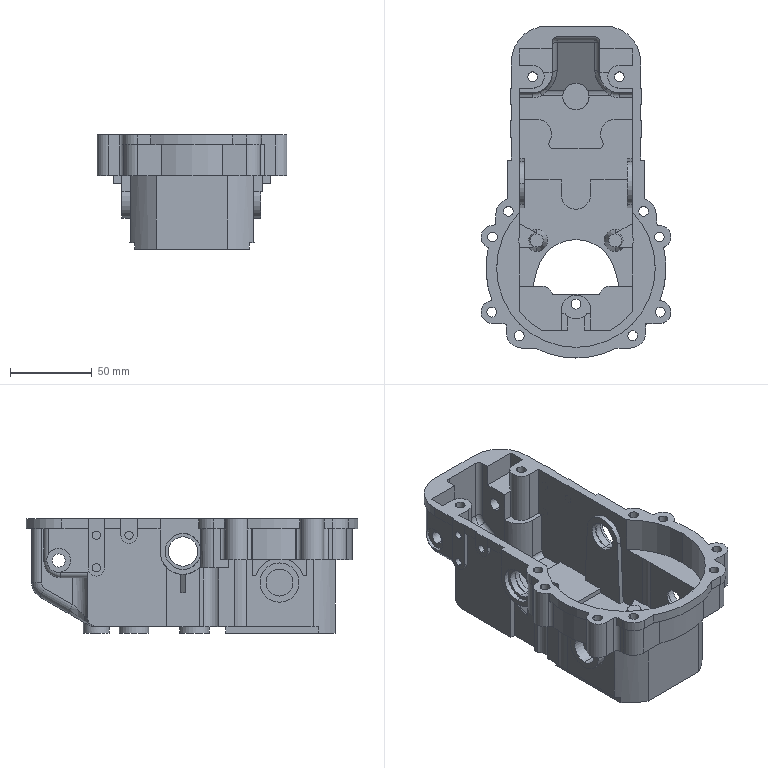Part | SolidWorks | features BaseBody 1 | 1 solid | 454 faces | box 116 x 203 x 70 mm | volume 236154 mm3 | plane 229 | cylinder 203 | torus 10 | spline 8 | cone 4 | commonest cylinder face diameters 6 x44 5 x22 18 x18 14 x15 10 x12 12 x10